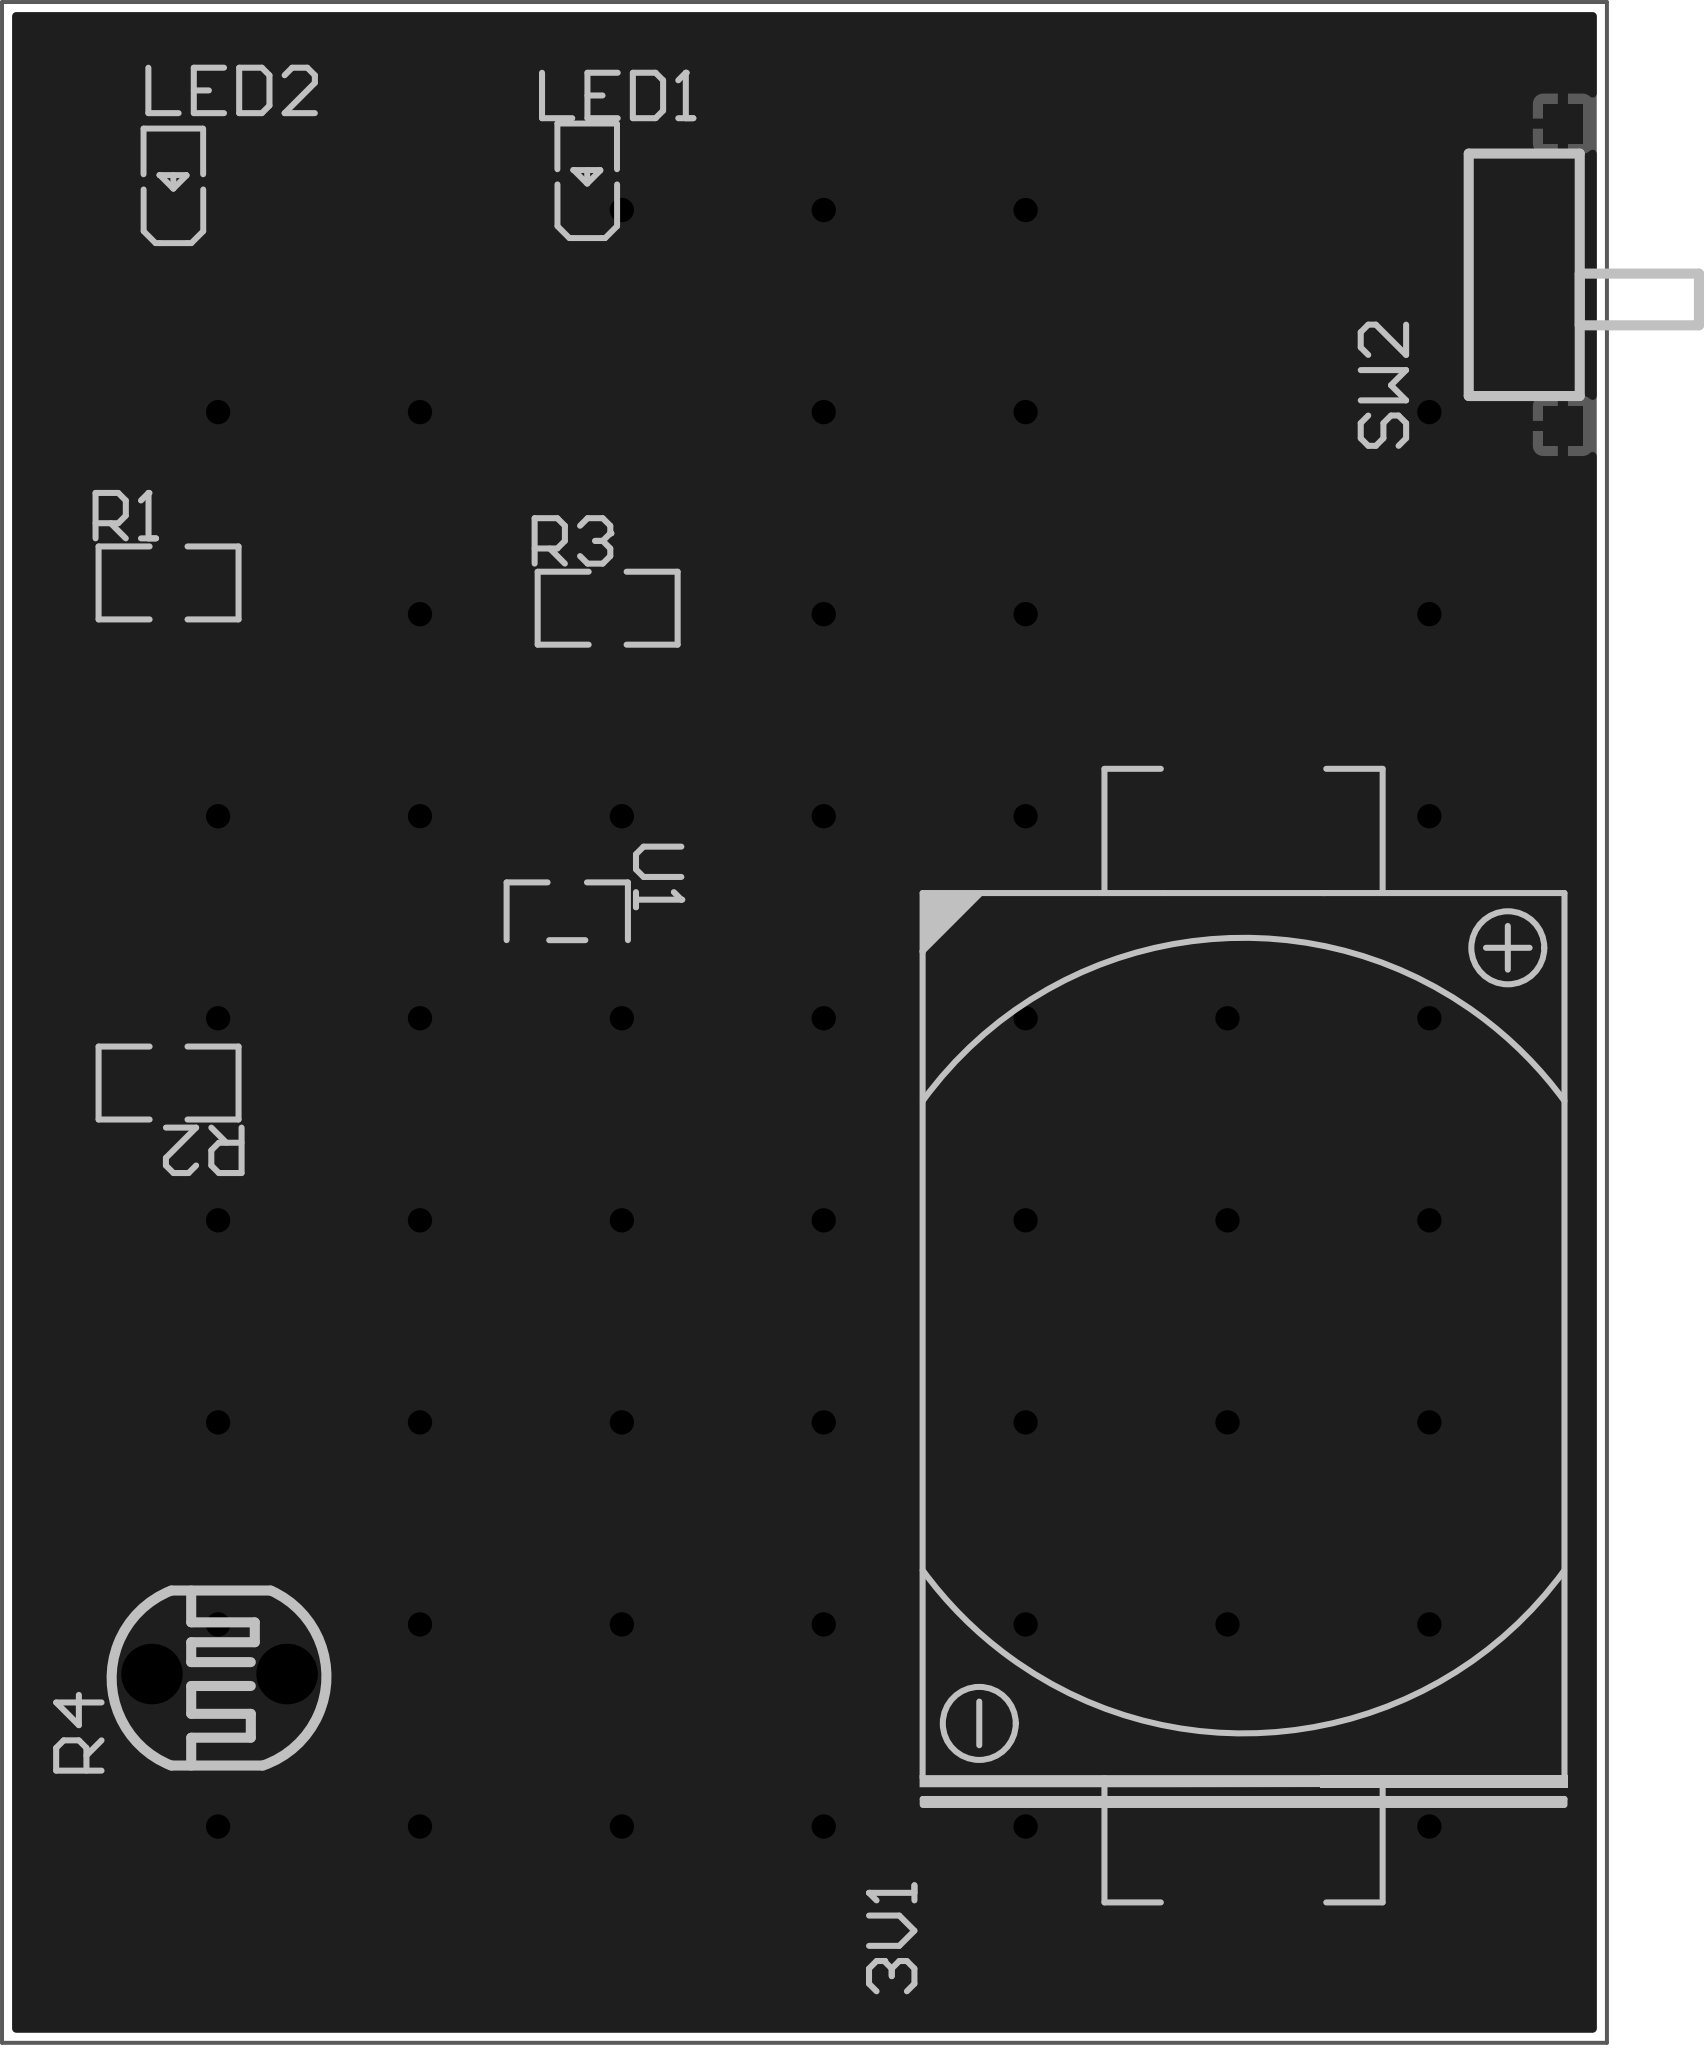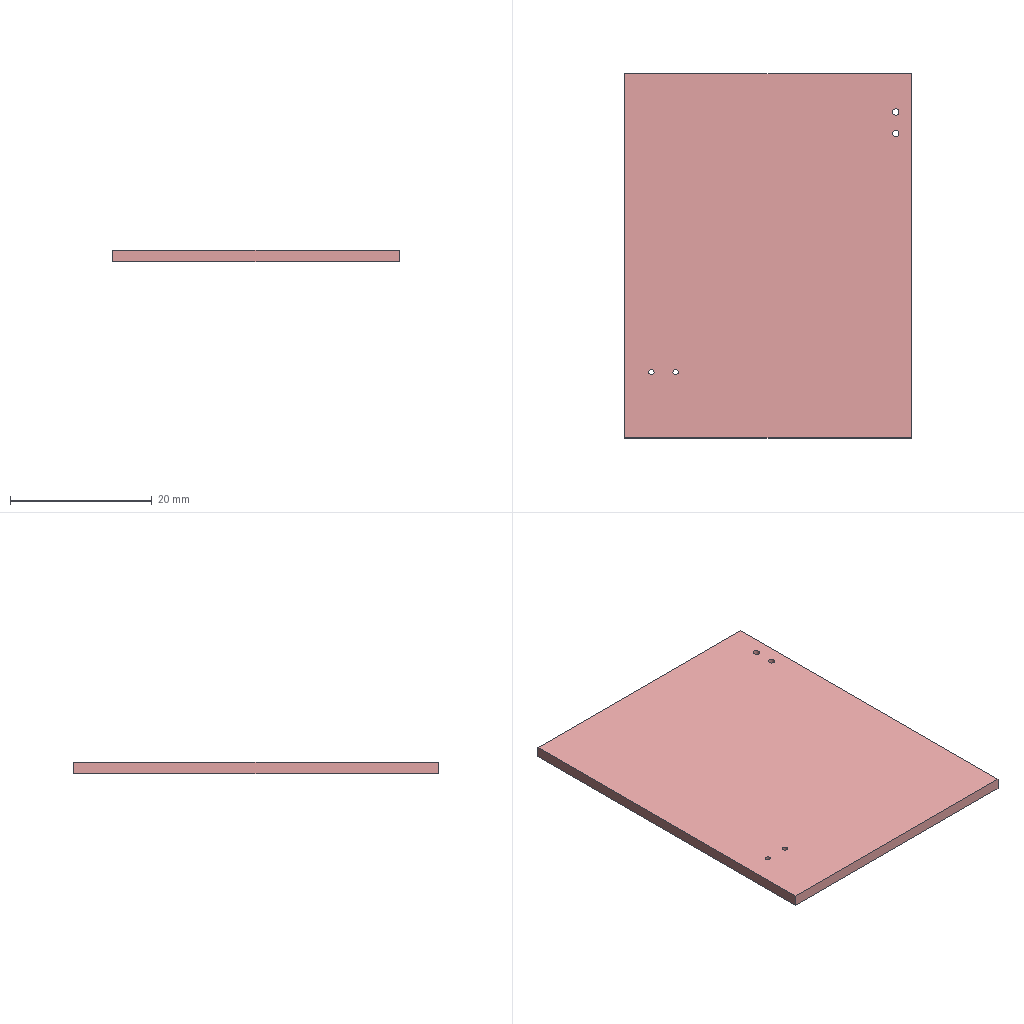Circuit board layout | Altium Designer | box 40.4 x 51.3 x 1.6 mm
Layer stack:
# Altium Designer layer stack of  (unit mm; dielectric type: 0 none, 1 core, 2 prepreg, 3 surface material)
index,name,kind,layer,copper_thickness_mm,dielectric_type,dielectric_thickness_mm,dielectric_material,dielectric_constant
0,Top Paste Mask Layer,other,,,,,,
1,Top Silkscreen Layer,other,,,,,,
2,Top Solder Mask Layer,dielectric,,,3,0.01,,3.3
3,Top Layer,copper,Top Layer,0.035,,,,
4,Dielectric1,dielectric,,,3,1.51,FR4,4.5
5,Bottom Layer,copper,Bottom Layer,0.035,,,,
6,Bottom Solder Mask Layer,dielectric,,,3,0.01,,3.3
7,Bottom Silkscreen Layer,other,,,,,,
8,Bottom Paste Mask Layer,other,,,,,,
# drill layer pairs: low layer,high layer
drill_pair,Top Layer,Bottom Layer
Part placement:
Designator,Comment,Layer,Footprint,Center-X(mm),Center-Y(mm),Rotation
3V1,,TopLayer,BAT-TH_CR2032-BS-6-1,115.57,100.711,90
LED1,NCD0603W1,TopLayer,LED0603-RD,99.06,129.794,90
LED2,NCD0603W1,TopLayer,LED0603-RD,88.646,129.667,90
R1,4.7kΩ,TopLayer,R0805,88.519,119.634,0
R2,1K,TopLayer,R0805,88.519,107.061,180
R3,100,TopLayer,R0805,99.568,118.999,0
R4,GL3516（5-10K）,TopLayer,RES-TH_L5.1-W4.3-P3.40-D0.5,89.789,92.202,90
SW2,SK-3296S-01-L1,TopLayer,SW-SMD_3P-P1.50_L2.7-W6.6,122.047,127.381,90
U1,S9013,TopLayer,SOT-23-3_L2.9-W1.3-P1.90-LS2.4-BR,98.552,111.379,270
Pad and via stacks:
# Altium Designer via and pad stacks of  (unit mm). Each distinct definition once, with the count of objects using it.
# via: kind,start_layer,end_layer,hole_mm,diameter_mm,mode(0 simple;1 top-mid-bottom;2 full stack),diameter_per_layer,count,example_net
# pad: kind,layer,hole_mm,hole_type(0 round;1 square;2 slot),plating,top_size,top_shape(1 round;2 rect;3 octagon;9 rounded rect),mid_size,bottom_size,mode,footprint,size_per_layer,count,example
pad,Top Layer,0,0,plated,4.2x3.8,2,4.2x3.8,4.2x3.8,0,BAT-TH_CR2032-BS-6-1,,2,3V1.1
pad,Top Layer,0,0,plated,0.8x0.8,2,0.8x0.8,0.8x0.8,0,LED0603-RD,,4,LED1.2
pad,Top Layer,0,0,plated,1.133x1.377,2,1.133x1.377,1.133x1.377,0,R0805,,6,R1.2
pad,Top Layer,0,0,plated,1x1,2,1x1,1x1,0,SW-SMD_3P-P1.50_L2.7-W6.6,,4,SW2.0
pad,Top Layer,0,0,plated,1x1.4,2,1x1.4,1x1.4,0,SW-SMD_3P-P1.50_L2.7-W6.6,,3,SW2.1
pad,Top Layer,0,0,plated,1.25x0.7,2,1.25x0.7,1.25x0.7,0,SOT-23-3_L2.9-W1.3-P1.90-LS2.4-BR,,3,U1.1
pad,Multi-Layer,0.762,0,plated,1.524x1.524,1,1.524x1.524,1.524x1.524,0,RES-TH_L5.1-W4.3-P3.40-D0.5,,2,R4.2
via,Top Layer,Bottom Layer,0.3048,0.61,0,,52,GND
Copper pours:
name,layer,net,type(0 solid;1 hatched;2 none)
Top Layer-GND,Top Layer,GND,0
Bottom Layer-GND,Bottom Layer,GND,0
Design rules, without the lines most boards share:
# Altium Designer design rules of  (exported by Altium Designer, unit mm)
# columns: name | kind | enabled | priority | scope1 | scope2 | descriptor | typed fields (field=value)
creepage | 65 | enabled | 1 | All | All | Creepage Distance Constraint =(0mil) (All),(All) |